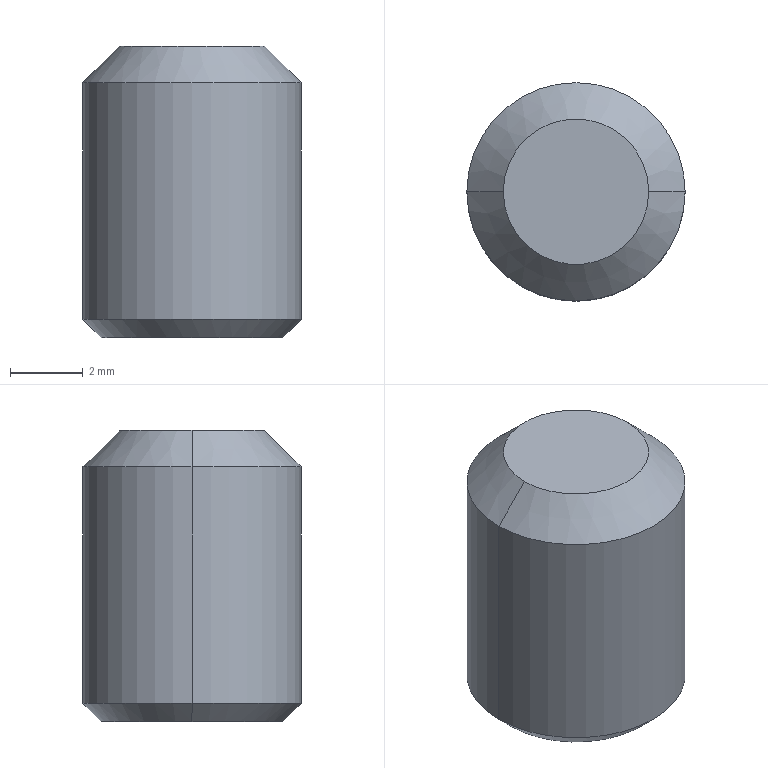Part | NX | features BREP 1 | 1 solid | 22 faces | box 6 x 6 x 8 mm | volume 197.963 mm3 | plane 14 | cone 6 | cylinder 2 | commonest cylinder face diameters 6 x2
STEP:
#1=CARTESIAN_POINT('',(0.,0.,2.866));
#2=VERTEX_POINT('',#1);
#3=CARTESIAN_POINT('',(-1.5,0.,2.));
#4=VERTEX_POINT('',#3);
#5=CARTESIAN_POINT('',(-1.5,0.,2.));
#6=DIRECTION('',(-0.866,0.,-0.5));
#7=VECTOR('',#6,1000.);
#8=LINE('',#5,#7);
#9=EDGE_CURVE('',#2,#4,#8,.T.);
#10=ORIENTED_EDGE('',*,*,#9,.F.);
#11=CARTESIAN_POINT('',(1.5,0.,2.));
#12=VERTEX_POINT('',#11);
#13=CARTESIAN_POINT('',(1.5,0.,2.));
#14=DIRECTION('',(0.866,0.,-0.5));
#15=VECTOR('',#14,1000.);
#16=LINE('',#13,#15);
#17=EDGE_CURVE('',#2,#12,#16,.T.);
#18=ORIENTED_EDGE('',*,*,#17,.T.);
#19=CARTESIAN_POINT('',(1.299,-0.75,2.));
#20=VERTEX_POINT('',#19);
#21=CARTESIAN_POINT('',(0.,0.,2.));
#22=DIRECTION('',(0.,0.,-1.));
#23=DIRECTION('',(-1.,0.,0.));
#24=AXIS2_PLACEMENT_3D('',#21,#22,#23);
#25=CIRCLE('',#24,1.5);
#26=EDGE_CURVE('',#12,#20,#25,.T.);
#27=ORIENTED_EDGE('',*,*,#26,.T.);
#28=CARTESIAN_POINT('',(0.,-1.5,2.));
#29=VERTEX_POINT('',#28);
#30=CARTESIAN_POINT('',(0.,0.,2.));
#31=DIRECTION('',(0.,0.,-1.));
#32=DIRECTION('',(-1.,0.,0.));
#33=AXIS2_PLACEMENT_3D('',#30,#31,#32);
#34=CIRCLE('',#33,1.5);
#35=EDGE_CURVE('',#20,#29,#34,.T.);
#36=ORIENTED_EDGE('',*,*,#35,.T.);
#37=CARTESIAN_POINT('',(-1.299,-0.75,2.));
#38=VERTEX_POINT('',#37);
#39=CARTESIAN_POINT('',(0.,0.,2.));
#40=DIRECTION('',(0.,0.,-1.));
#41=DIRECTION('',(-1.,0.,0.));
#42=AXIS2_PLACEMENT_3D('',#39,#40,#41);
#43=CIRCLE('',#42,1.5);
#44=EDGE_CURVE('',#29,#38,#43,.T.);
#45=ORIENTED_EDGE('',*,*,#44,.T.);
#46=CARTESIAN_POINT('',(0.,0.,2.));
#47=DIRECTION('',(0.,0.,-1.));
#48=DIRECTION('',(-1.,0.,0.));
#49=AXIS2_PLACEMENT_3D('',#46,#47,#48);
#50=CIRCLE('',#49,1.5);
#51=EDGE_CURVE('',#38,#4,#50,.T.);
#52=ORIENTED_EDGE('',*,*,#51,.T.);
#53=EDGE_LOOP('',(#10,#18,#27,#36,#45,#52));
#54=FACE_BOUND('',#53,.T.);
#55=CARTESIAN_POINT('',(0.,0.,2.));
#56=DIRECTION('',(0.,0.,-1.));
#57=DIRECTION('',(-1.,0.,0.));
#58=AXIS2_PLACEMENT_3D('',#55,#56,#57);
#59=CONICAL_SURFACE('',#58,1.5,1.047);
#60=ADVANCED_FACE('',(#54),#59,.F.);
#61=CARTESIAN_POINT('',(2.,0.,8.));
#62=VERTEX_POINT('',#61);
#63=CARTESIAN_POINT('',(-2.,0.,8.));
#64=VERTEX_POINT('',#63);
#65=CARTESIAN_POINT('',(0.,0.,8.));
#66=DIRECTION('',(0.,0.,1.));
#67=DIRECTION('',(1.,0.,0.));
#68=AXIS2_PLACEMENT_3D('',#65,#66,#67);
#69=CIRCLE('',#68,2.);
#70=EDGE_CURVE('',#62,#64,#69,.T.);
#71=ORIENTED_EDGE('',*,*,#70,.F.);
#72=CARTESIAN_POINT('',(3.,0.,7.));
#73=VERTEX_POINT('',#72);
#74=CARTESIAN_POINT('',(2.,0.,8.));
#75=DIRECTION('',(0.7071,0.,-0.7071));
#76=VECTOR('',#75,1000.);
#77=LINE('',#74,#76);
#78=EDGE_CURVE('',#62,#73,#77,.T.);
#79=ORIENTED_EDGE('',*,*,#78,.T.);
#80=CARTESIAN_POINT('',(-3.,0.,7.));
#81=VERTEX_POINT('',#80);
#82=CARTESIAN_POINT('',(0.,0.,7.));
#83=DIRECTION('',(0.,0.,-1.));
#84=DIRECTION('',(1.,0.,0.));
#85=AXIS2_PLACEMENT_3D('',#82,#83,#84);
#86=CIRCLE('',#85,3.);
#87=EDGE_CURVE('',#81,#73,#86,.T.);
#88=ORIENTED_EDGE('',*,*,#87,.F.);
#89=CARTESIAN_POINT('',(-2.,0.,8.));
#90=DIRECTION('',(-0.7071,0.,-0.7071));
#91=VECTOR('',#90,1000.);
#92=LINE('',#89,#91);
#93=EDGE_CURVE('',#64,#81,#92,.T.);
#94=ORIENTED_EDGE('',*,*,#93,.F.);
#95=EDGE_LOOP('',(#71,#79,#88,#94));
#96=FACE_BOUND('',#95,.T.);
#97=CARTESIAN_POINT('',(0.,0.,8.));
#98=DIRECTION('',(0.,0.,-1.));
#99=DIRECTION('',(-1.,0.,0.));
#100=AXIS2_PLACEMENT_3D('',#97,#98,#99);
#101=CONICAL_SURFACE('',#100,2.,0.7854);
#102=ADVANCED_FACE('',(#96),#101,.T.);
#103=CARTESIAN_POINT('',(-2.5,0.,0.));
#104=VERTEX_POINT('',#103);
#105=CARTESIAN_POINT('',(2.5,0.,0.));
#106=VERTEX_POINT('',#105);
#107=CARTESIAN_POINT('',(0.,0.,0.));
#108=DIRECTION('',(0.,0.,-1.));
#109=DIRECTION('',(1.,0.,0.));
#110=AXIS2_PLACEMENT_3D('',#107,#108,#109);
#111=CIRCLE('',#110,2.5);
#112=EDGE_CURVE('',#104,#106,#111,.T.);
#113=ORIENTED_EDGE('',*,*,#112,.F.);
#114=CARTESIAN_POINT('',(-3.,0.,0.5));
#115=VERTEX_POINT('',#114);
#116=CARTESIAN_POINT('',(-3.,0.,0.5));
#117=DIRECTION('',(-0.7071,0.,0.7071));
#118=VECTOR('',#117,1000.);
#119=LINE('',#116,#118);
#120=EDGE_CURVE('',#115,#104,#119,.F.);
#121=ORIENTED_EDGE('',*,*,#120,.F.);
#122=CARTESIAN_POINT('',(3.,0.,0.5));
#123=VERTEX_POINT('',#122);
#124=CARTESIAN_POINT('',(0.,0.,0.5));
#125=DIRECTION('',(0.,0.,1.));
#126=DIRECTION('',(1.,0.,0.));
#127=AXIS2_PLACEMENT_3D('',#124,#125,#126);
#128=CIRCLE('',#127,3.);
#129=EDGE_CURVE('',#123,#115,#128,.T.);
#130=ORIENTED_EDGE('',*,*,#129,.F.);
#131=CARTESIAN_POINT('',(3.,0.,0.5));
#132=DIRECTION('',(0.7071,0.,0.7071));
#133=VECTOR('',#132,1000.);
#134=LINE('',#131,#133);
#135=EDGE_CURVE('',#123,#106,#134,.F.);
#136=ORIENTED_EDGE('',*,*,#135,.T.);
#137=EDGE_LOOP('',(#113,#121,#130,#136));
#138=FACE_BOUND('',#137,.T.);
#139=CARTESIAN_POINT('',(0.,0.,0.5));
#140=DIRECTION('',(0.,0.,1.));
#141=DIRECTION('',(1.,0.,0.));
#142=AXIS2_PLACEMENT_3D('',#139,#140,#141);
#143=CONICAL_SURFACE('',#142,3.,0.7854);
#144=ADVANCED_FACE('',(#138),#143,.T.);
#145=ORIENTED_EDGE('',*,*,#87,.T.);
#146=CARTESIAN_POINT('',(3.,0.,8.));
#147=DIRECTION('',(0.,0.,-1.));
#148=VECTOR('',#147,1000.);
#149=LINE('',#146,#148);
#150=EDGE_CURVE('',#73,#123,#149,.T.);
#151=ORIENTED_EDGE('',*,*,#150,.T.);
#152=ORIENTED_EDGE('',*,*,#129,.T.);
#153=CARTESIAN_POINT('',(-3.,0.,8.));
#154=DIRECTION('',(0.,0.,-1.));
#155=VECTOR('',#154,1000.);
#156=LINE('',#153,#155);
#157=EDGE_CURVE('',#81,#115,#156,.T.);
#158=ORIENTED_EDGE('',*,*,#157,.F.);
#159=EDGE_LOOP('',(#145,#151,#152,#158));
#160=FACE_BOUND('',#159,.T.);
#161=CARTESIAN_POINT('',(0.,0.,8.));
#162=DIRECTION('',(0.,0.,-1.));
#163=DIRECTION('',(-1.,0.,0.));
#164=AXIS2_PLACEMENT_3D('',#161,#162,#163);
#165=CYLINDRICAL_SURFACE('',#164,3.);
#166=ADVANCED_FACE('',(#160),#165,.T.);
#167=CARTESIAN_POINT('',(-1.299,0.75,2.));
#168=VERTEX_POINT('',#167);
#169=CARTESIAN_POINT('',(0.,1.5,2.));
#170=VERTEX_POINT('',#169);
#171=CARTESIAN_POINT('',(0.,0.,2.));
#172=DIRECTION('',(0.,0.,-1.));
#173=DIRECTION('',(-1.,0.,0.));
#174=AXIS2_PLACEMENT_3D('',#171,#172,#173);
#175=CIRCLE('',#174,1.5);
#176=EDGE_CURVE('',#168,#170,#175,.T.);
#177=ORIENTED_EDGE('',*,*,#176,.F.);
#178=CARTESIAN_POINT('',(-0.866,1.5,2.));
#179=VERTEX_POINT('',#178);
#180=CARTESIAN_POINT('',(-1.732,0.,2.));
#181=DIRECTION('',(0.5,0.866,0.));
#182=VECTOR('',#181,1000.);
#183=LINE('',#180,#182);
#184=EDGE_CURVE('',#168,#179,#183,.T.);
#185=ORIENTED_EDGE('',*,*,#184,.T.);
#186=CARTESIAN_POINT('',(-0.866,1.5,2.));
#187=DIRECTION('',(1.,0.,0.));
#188=VECTOR('',#187,1000.);
#189=LINE('',#186,#188);
#190=EDGE_CURVE('',#179,#170,#189,.T.);
#191=ORIENTED_EDGE('',*,*,#190,.T.);
#192=EDGE_LOOP('',(#177,#185,#191));
#193=FACE_BOUND('',#192,.T.);
#194=CARTESIAN_POINT('',(0.,0.,2.));
#195=DIRECTION('',(0.,0.,-1.));
#196=DIRECTION('',(0.,-1.,0.));
#197=AXIS2_PLACEMENT_3D('',#194,#195,#196);
#198=PLANE('',#197);
#199=ADVANCED_FACE('',(#193),#198,.T.);
#200=CARTESIAN_POINT('',(1.299,0.75,2.));
#201=VERTEX_POINT('',#200);
#202=CARTESIAN_POINT('',(0.,0.,2.));
#203=DIRECTION('',(0.,0.,-1.));
#204=DIRECTION('',(-1.,0.,0.));
#205=AXIS2_PLACEMENT_3D('',#202,#203,#204);
#206=CIRCLE('',#205,1.5);
#207=EDGE_CURVE('',#170,#201,#206,.T.);
#208=ORIENTED_EDGE('',*,*,#207,.F.);
#209=CARTESIAN_POINT('',(0.866,1.5,2.));
#210=VERTEX_POINT('',#209);
#211=CARTESIAN_POINT('',(-0.866,1.5,2.));
#212=DIRECTION('',(1.,0.,0.));
#213=VECTOR('',#212,1000.);
#214=LINE('',#211,#213);
#215=EDGE_CURVE('',#170,#210,#214,.T.);
#216=ORIENTED_EDGE('',*,*,#215,.T.);
#217=CARTESIAN_POINT('',(0.866,1.5,2.));
#218=DIRECTION('',(0.5,-0.866,0.));
#219=VECTOR('',#218,1000.);
#220=LINE('',#217,#219);
#221=EDGE_CURVE('',#210,#201,#220,.T.);
#222=ORIENTED_EDGE('',*,*,#221,.T.);
#223=EDGE_LOOP('',(#208,#216,#222));
#224=FACE_BOUND('',#223,.T.);
#225=CARTESIAN_POINT('',(0.,0.,2.));
#226=DIRECTION('',(0.,0.,-1.));
#227=DIRECTION('',(0.,-1.,0.));
#228=AXIS2_PLACEMENT_3D('',#225,#226,#227);
#229=PLANE('',#228);
#230=ADVANCED_FACE('',(#224),#229,.T.);
#231=CARTESIAN_POINT('',(0.,0.,2.));
#232=DIRECTION('',(0.,0.,-1.));
#233=DIRECTION('',(-1.,0.,0.));
#234=AXIS2_PLACEMENT_3D('',#231,#232,#233);
#235=CIRCLE('',#234,1.5);
#236=EDGE_CURVE('',#201,#12,#235,.T.);
#237=ORIENTED_EDGE('',*,*,#236,.F.);
#238=CARTESIAN_POINT('',(1.732,0.,2.));
#239=VERTEX_POINT('',#238);
#240=CARTESIAN_POINT('',(0.866,1.5,2.));
#241=DIRECTION('',(0.5,-0.866,0.));
#242=VECTOR('',#241,1000.);
#243=LINE('',#240,#242);
#244=EDGE_CURVE('',#201,#239,#243,.T.);
#245=ORIENTED_EDGE('',*,*,#244,.T.);
#246=CARTESIAN_POINT('',(1.732,0.,2.));
#247=DIRECTION('',(-0.5,-0.866,0.));
#248=VECTOR('',#247,1000.);
#249=LINE('',#246,#248);
#250=EDGE_CURVE('',#239,#20,#249,.T.);
#251=ORIENTED_EDGE('',*,*,#250,.T.);
#252=ORIENTED_EDGE('',*,*,#26,.F.);
#253=EDGE_LOOP('',(#237,#245,#251,#252));
#254=FACE_BOUND('',#253,.T.);
#255=CARTESIAN_POINT('',(0.,0.,2.));
#256=DIRECTION('',(0.,0.,-1.));
#257=DIRECTION('',(0.,-1.,0.));
#258=AXIS2_PLACEMENT_3D('',#255,#256,#257);
#259=PLANE('',#258);
#260=ADVANCED_FACE('',(#254),#259,.T.);
#261=ORIENTED_EDGE('',*,*,#35,.F.);
#262=CARTESIAN_POINT('',(0.866,-1.5,2.));
#263=VERTEX_POINT('',#262);
#264=CARTESIAN_POINT('',(1.732,0.,2.));
#265=DIRECTION('',(-0.5,-0.866,0.));
#266=VECTOR('',#265,1000.);
#267=LINE('',#264,#266);
#268=EDGE_CURVE('',#20,#263,#267,.T.);
#269=ORIENTED_EDGE('',*,*,#268,.T.);
#270=CARTESIAN_POINT('',(0.866,-1.5,2.));
#271=DIRECTION('',(-1.,0.,0.));
#272=VECTOR('',#271,1000.);
#273=LINE('',#270,#272);
#274=EDGE_CURVE('',#263,#29,#273,.T.);
#275=ORIENTED_EDGE('',*,*,#274,.T.);
#276=EDGE_LOOP('',(#261,#269,#275));
#277=FACE_BOUND('',#276,.T.);
#278=CARTESIAN_POINT('',(0.,0.,2.));
#279=DIRECTION('',(0.,0.,-1.));
#280=DIRECTION('',(0.,-1.,0.));
#281=AXIS2_PLACEMENT_3D('',#278,#279,#280);
#282=PLANE('',#281);
#283=ADVANCED_FACE('',(#277),#282,.T.);
#284=ORIENTED_EDGE('',*,*,#44,.F.);
#285=CARTESIAN_POINT('',(-0.866,-1.5,2.));
#286=VERTEX_POINT('',#285);
#287=CARTESIAN_POINT('',(0.866,-1.5,2.));
#288=DIRECTION('',(-1.,0.,0.));
#289=VECTOR('',#288,1000.);
#290=LINE('',#287,#289);
#291=EDGE_CURVE('',#29,#286,#290,.T.);
#292=ORIENTED_EDGE('',*,*,#291,.T.);
#293=CARTESIAN_POINT('',(-0.866,-1.5,2.));
#294=DIRECTION('',(-0.5,0.866,0.));
#295=VECTOR('',#294,1000.);
#296=LINE('',#293,#295);
#297=EDGE_CURVE('',#286,#38,#296,.T.);
#298=ORIENTED_EDGE('',*,*,#297,.T.);
#299=EDGE_LOOP('',(#284,#292,#298));
#300=FACE_BOUND('',#299,.T.);
#301=CARTESIAN_POINT('',(0.,0.,2.));
#302=DIRECTION('',(0.,0.,-1.));
#303=DIRECTION('',(0.,-1.,0.));
#304=AXIS2_PLACEMENT_3D('',#301,#302,#303);
#305=PLANE('',#304);
#306=ADVANCED_FACE('',(#300),#305,.T.);
#307=ORIENTED_EDGE('',*,*,#150,.F.);
#308=CARTESIAN_POINT('',(0.,0.,7.));
#309=DIRECTION('',(0.,0.,-1.));
#310=DIRECTION('',(1.,0.,0.));
#311=AXIS2_PLACEMENT_3D('',#308,#309,#310);
#312=CIRCLE('',#311,3.);
#313=EDGE_CURVE('',#73,#81,#312,.T.);
#314=ORIENTED_EDGE('',*,*,#313,.T.);
#315=ORIENTED_EDGE('',*,*,#157,.T.);
#316=CARTESIAN_POINT('',(0.,0.,0.5));
#317=DIRECTION('',(0.,0.,1.));
#318=DIRECTION('',(1.,0.,0.));
#319=AXIS2_PLACEMENT_3D('',#316,#317,#318);
#320=CIRCLE('',#319,3.);
#321=EDGE_CURVE('',#115,#123,#320,.T.);
#322=ORIENTED_EDGE('',*,*,#321,.T.);
#323=EDGE_LOOP('',(#307,#314,#315,#322));
#324=FACE_BOUND('',#323,.T.);
#325=CARTESIAN_POINT('',(0.,0.,8.));
#326=DIRECTION('',(0.,0.,-1.));
#327=DIRECTION('',(-1.,0.,0.));
#328=AXIS2_PLACEMENT_3D('',#325,#326,#327);
#329=CYLINDRICAL_SURFACE('',#328,3.);
#330=ADVANCED_FACE('',(#324),#329,.T.);
#331=CARTESIAN_POINT('',(0.,0.,8.));
#332=DIRECTION('',(0.,0.,1.));
#333=DIRECTION('',(1.,0.,0.));
#334=AXIS2_PLACEMENT_3D('',#331,#332,#333);
#335=CIRCLE('',#334,2.);
#336=EDGE_CURVE('',#64,#62,#335,.T.);
#337=ORIENTED_EDGE('',*,*,#336,.T.);
#338=ORIENTED_EDGE('',*,*,#70,.T.);
#339=EDGE_LOOP('',(#337,#338));
#340=FACE_BOUND('',#339,.T.);
#341=CARTESIAN_POINT('',(0.,0.,8.));
#342=DIRECTION('',(0.,0.,1.));
#343=DIRECTION('',(1.,0.,0.));
#344=AXIS2_PLACEMENT_3D('',#341,#342,#343);
#345=PLANE('',#344);
#346=ADVANCED_FACE('',(#340),#345,.T.);
#347=CARTESIAN_POINT('',(0.,0.,0.));
#348=DIRECTION('',(0.,0.,-1.));
#349=DIRECTION('',(1.,0.,0.));
#350=AXIS2_PLACEMENT_3D('',#347,#348,#349);
#351=CIRCLE('',#350,2.5);
#352=EDGE_CURVE('',#106,#104,#351,.T.);
#353=ORIENTED_EDGE('',*,*,#352,.T.);
#354=ORIENTED_EDGE('',*,*,#112,.T.);
#355=EDGE_LOOP('',(#353,#354));
#356=FACE_BOUND('',#355,.T.);
#357=CARTESIAN_POINT('',(-0.866,1.5,0.));
#358=VERTEX_POINT('',#357);
#359=CARTESIAN_POINT('',(0.866,1.5,0.));
#360=VERTEX_POINT('',#359);
#361=CARTESIAN_POINT('',(-0.866,1.5,0.));
#362=DIRECTION('',(1.,0.,0.));
#363=VECTOR('',#362,1000.);
#364=LINE('',#361,#363);
#365=EDGE_CURVE('',#358,#360,#364,.T.);
#366=ORIENTED_EDGE('',*,*,#365,.F.);
#367=CARTESIAN_POINT('',(-1.732,0.,0.));
#368=VERTEX_POINT('',#367);
#369=CARTESIAN_POINT('',(-1.732,0.,0.));
#370=DIRECTION('',(0.5,0.866,0.));
#371=VECTOR('',#370,1000.);
#372=LINE('',#369,#371);
#373=EDGE_CURVE('',#368,#358,#372,.T.);
#374=ORIENTED_EDGE('',*,*,#373,.F.);
#375=CARTESIAN_POINT('',(-0.866,-1.5,0.));
#376=VERTEX_POINT('',#375);
#377=CARTESIAN_POINT('',(-0.866,-1.5,0.));
#378=DIRECTION('',(-0.5,0.866,0.));
#379=VECTOR('',#378,1000.);
#380=LINE('',#377,#379);
#381=EDGE_CURVE('',#376,#368,#380,.T.);
#382=ORIENTED_EDGE('',*,*,#381,.F.);
#383=CARTESIAN_POINT('',(0.866,-1.5,0.));
#384=VERTEX_POINT('',#383);
#385=CARTESIAN_POINT('',(0.866,-1.5,0.));
#386=DIRECTION('',(-1.,0.,0.));
#387=VECTOR('',#386,1000.);
#388=LINE('',#385,#387);
#389=EDGE_CURVE('',#384,#376,#388,.T.);
#390=ORIENTED_EDGE('',*,*,#389,.F.);
#391=CARTESIAN_POINT('',(1.732,0.,0.));
#392=VERTEX_POINT('',#391);
#393=CARTESIAN_POINT('',(1.732,0.,0.));
#394=DIRECTION('',(-0.5,-0.866,0.));
#395=VECTOR('',#394,1000.);
#396=LINE('',#393,#395);
#397=EDGE_CURVE('',#392,#384,#396,.T.);
#398=ORIENTED_EDGE('',*,*,#397,.F.);
#399=CARTESIAN_POINT('',(0.866,1.5,0.));
#400=DIRECTION('',(0.5,-0.866,0.));
#401=VECTOR('',#400,1000.);
#402=LINE('',#399,#401);
#403=EDGE_CURVE('',#360,#392,#402,.T.);
#404=ORIENTED_EDGE('',*,*,#403,.F.);
#405=EDGE_LOOP('',(#366,#374,#382,#390,#398,#404));
#406=FACE_BOUND('',#405,.T.);
#407=CARTESIAN_POINT('',(0.,0.,0.));
#408=DIRECTION('',(0.,0.,1.));
#409=DIRECTION('',(1.,0.,0.));
#410=AXIS2_PLACEMENT_3D('',#407,#408,#409);
#411=PLANE('',#410);
#412=ADVANCED_FACE('',(#356,#406),#411,.F.);
#413=ORIENTED_EDGE('',*,*,#120,.T.);
#414=ORIENTED_EDGE('',*,*,#352,.F.);
#415=ORIENTED_EDGE('',*,*,#135,.F.);
#416=ORIENTED_EDGE('',*,*,#321,.F.);
#417=EDGE_LOOP('',(#413,#414,#415,#416));
#418=FACE_BOUND('',#417,.T.);
#419=CARTESIAN_POINT('',(0.,0.,0.5));
#420=DIRECTION('',(0.,0.,1.));
#421=DIRECTION('',(1.,0.,0.));
#422=AXIS2_PLACEMENT_3D('',#419,#420,#421);
#423=CONICAL_SURFACE('',#422,3.,0.7854);
#424=ADVANCED_FACE('',(#418),#423,.T.);
#425=ORIENTED_EDGE('',*,*,#78,.F.);
#426=ORIENTED_EDGE('',*,*,#336,.F.);
#427=ORIENTED_EDGE('',*,*,#93,.T.);
#428=ORIENTED_EDGE('',*,*,#313,.F.);
#429=EDGE_LOOP('',(#425,#426,#427,#428));
#430=FACE_BOUND('',#429,.T.);
#431=CARTESIAN_POINT('',(0.,0.,8.));
#432=DIRECTION('',(0.,0.,-1.));
#433=DIRECTION('',(-1.,0.,0.));
#434=AXIS2_PLACEMENT_3D('',#431,#432,#433);
#435=CONICAL_SURFACE('',#434,2.,0.7854);
#436=ADVANCED_FACE('',(#430),#435,.T.);
#437=ORIENTED_EDGE('',*,*,#373,.T.);
#438=CARTESIAN_POINT('',(-0.866,1.5,2.));
#439=DIRECTION('',(0.,0.,-1.));
#440=VECTOR('',#439,1000.);
#441=LINE('',#438,#440);
#442=EDGE_CURVE('',#179,#358,#441,.T.);
#443=ORIENTED_EDGE('',*,*,#442,.F.);
#444=ORIENTED_EDGE('',*,*,#184,.F.);
#445=CARTESIAN_POINT('',(-1.732,0.,2.));
#446=VERTEX_POINT('',#445);
#447=CARTESIAN_POINT('',(-1.732,0.,2.));
#448=DIRECTION('',(0.5,0.866,0.));
#449=VECTOR('',#448,1000.);
#450=LINE('',#447,#449);
#451=EDGE_CURVE('',#446,#168,#450,.T.);
#452=ORIENTED_EDGE('',*,*,#451,.F.);
#453=CARTESIAN_POINT('',(-1.732,0.,2.));
#454=DIRECTION('',(0.,0.,-1.));
#455=VECTOR('',#454,1000.);
#456=LINE('',#453,#455);
#457=EDGE_CURVE('',#446,#368,#456,.T.);
#458=ORIENTED_EDGE('',*,*,#457,.T.);
#459=EDGE_LOOP('',(#437,#443,#444,#452,#458));
#460=FACE_BOUND('',#459,.T.);
#461=CARTESIAN_POINT('',(-1.732,0.,2.));
#462=DIRECTION('',(-0.866,0.5,0.));
#463=DIRECTION('',(0.,0.,1.));
#464=AXIS2_PLACEMENT_3D('',#461,#462,#463);
#465=PLANE('',#464);
#466=ADVANCED_FACE('',(#460),#465,.F.);
#467=ORIENTED_EDGE('',*,*,#381,.T.);
#468=ORIENTED_EDGE('',*,*,#457,.F.);
#469=CARTESIAN_POINT('',(-0.866,-1.5,2.));
#470=DIRECTION('',(-0.5,0.866,0.));
#471=VECTOR('',#470,1000.);
#472=LINE('',#469,#471);
#473=EDGE_CURVE('',#38,#446,#472,.T.);
#474=ORIENTED_EDGE('',*,*,#473,.F.);
#475=ORIENTED_EDGE('',*,*,#297,.F.);
#476=CARTESIAN_POINT('',(-0.866,-1.5,2.));
#477=DIRECTION('',(0.,0.,-1.));
#478=VECTOR('',#477,1000.);
#479=LINE('',#476,#478);
#480=EDGE_CURVE('',#286,#376,#479,.T.);
#481=ORIENTED_EDGE('',*,*,#480,.T.);
#482=EDGE_LOOP('',(#467,#468,#474,#475,#481));
#483=FACE_BOUND('',#482,.T.);
#484=CARTESIAN_POINT('',(-0.866,-1.5,2.));
#485=DIRECTION('',(-0.866,-0.5,0.));
#486=DIRECTION('',(-0.5,0.866,0.));
#487=AXIS2_PLACEMENT_3D('',#484,#485,#486);
#488=PLANE('',#487);
#489=ADVANCED_FACE('',(#483),#488,.F.);
#490=ORIENTED_EDGE('',*,*,#389,.T.);
#491=ORIENTED_EDGE('',*,*,#480,.F.);
#492=ORIENTED_EDGE('',*,*,#291,.F.);
#493=ORIENTED_EDGE('',*,*,#274,.F.);
#494=CARTESIAN_POINT('',(0.866,-1.5,2.));
#495=DIRECTION('',(0.,0.,-1.));
#496=VECTOR('',#495,1000.);
#497=LINE('',#494,#496);
#498=EDGE_CURVE('',#263,#384,#497,.T.);
#499=ORIENTED_EDGE('',*,*,#498,.T.);
#500=EDGE_LOOP('',(#490,#491,#492,#493,#499));
#501=FACE_BOUND('',#500,.T.);
#502=CARTESIAN_POINT('',(0.866,-1.5,2.));
#503=DIRECTION('',(0.,-1.,0.));
#504=DIRECTION('',(0.,0.,-1.));
#505=AXIS2_PLACEMENT_3D('',#502,#503,#504);
#506=PLANE('',#505);
#507=ADVANCED_FACE('',(#501),#506,.F.);
#508=ORIENTED_EDGE('',*,*,#397,.T.);
#509=ORIENTED_EDGE('',*,*,#498,.F.);
#510=ORIENTED_EDGE('',*,*,#268,.F.);
#511=ORIENTED_EDGE('',*,*,#250,.F.);
#512=CARTESIAN_POINT('',(1.732,0.,2.));
#513=DIRECTION('',(0.,0.,-1.));
#514=VECTOR('',#513,1000.);
#515=LINE('',#512,#514);
#516=EDGE_CURVE('',#239,#392,#515,.T.);
#517=ORIENTED_EDGE('',*,*,#516,.T.);
#518=EDGE_LOOP('',(#508,#509,#510,#511,#517));
#519=FACE_BOUND('',#518,.T.);
#520=CARTESIAN_POINT('',(1.732,0.,2.));
#521=DIRECTION('',(0.866,-0.5,0.));
#522=DIRECTION('',(0.,0.,-1.));
#523=AXIS2_PLACEMENT_3D('',#520,#521,#522);
#524=PLANE('',#523);
#525=ADVANCED_FACE('',(#519),#524,.F.);
#526=ORIENTED_EDGE('',*,*,#403,.T.);
#527=ORIENTED_EDGE('',*,*,#516,.F.);
#528=ORIENTED_EDGE('',*,*,#244,.F.);
#529=ORIENTED_EDGE('',*,*,#221,.F.);
#530=CARTESIAN_POINT('',(0.866,1.5,2.));
#531=DIRECTION('',(0.,0.,-1.));
#532=VECTOR('',#531,1000.);
#533=LINE('',#530,#532);
#534=EDGE_CURVE('',#210,#360,#533,.T.);
#535=ORIENTED_EDGE('',*,*,#534,.T.);
#536=EDGE_LOOP('',(#526,#527,#528,#529,#535));
#537=FACE_BOUND('',#536,.T.);
#538=CARTESIAN_POINT('',(0.866,1.5,2.));
#539=DIRECTION('',(0.866,0.5,0.));
#540=DIRECTION('',(0.,0.,-1.));
#541=AXIS2_PLACEMENT_3D('',#538,#539,#540);
#542=PLANE('',#541);
#543=ADVANCED_FACE('',(#537),#542,.F.);
#544=ORIENTED_EDGE('',*,*,#365,.T.);
#545=ORIENTED_EDGE('',*,*,#534,.F.);
#546=ORIENTED_EDGE('',*,*,#215,.F.);
#547=ORIENTED_EDGE('',*,*,#190,.F.);
#548=ORIENTED_EDGE('',*,*,#442,.T.);
#549=EDGE_LOOP('',(#544,#545,#546,#547,#548));
#550=FACE_BOUND('',#549,.T.);
#551=CARTESIAN_POINT('',(-0.866,1.5,2.));
#552=DIRECTION('',(0.,1.,0.));
#553=DIRECTION('',(1.,0.,0.));
#554=AXIS2_PLACEMENT_3D('',#551,#552,#553);
#555=PLANE('',#554);
#556=ADVANCED_FACE('',(#550),#555,.F.);
#557=ORIENTED_EDGE('',*,*,#51,.F.);
#558=ORIENTED_EDGE('',*,*,#473,.T.);
#559=ORIENTED_EDGE('',*,*,#451,.T.);
#560=CARTESIAN_POINT('',(0.,0.,2.));
#561=DIRECTION('',(0.,0.,-1.));
#562=DIRECTION('',(-1.,0.,0.));
#563=AXIS2_PLACEMENT_3D('',#560,#561,#562);
#564=CIRCLE('',#563,1.5);
#565=EDGE_CURVE('',#4,#168,#564,.T.);
#566=ORIENTED_EDGE('',*,*,#565,.F.);
#567=EDGE_LOOP('',(#557,#558,#559,#566));
#568=FACE_BOUND('',#567,.T.);
#569=CARTESIAN_POINT('',(0.,0.,2.));
#570=DIRECTION('',(0.,0.,-1.));
#571=DIRECTION('',(0.,-1.,0.));
#572=AXIS2_PLACEMENT_3D('',#569,#570,#571);
#573=PLANE('',#572);
#574=ADVANCED_FACE('',(#568),#573,.T.);
#575=ORIENTED_EDGE('',*,*,#17,.F.);
#576=ORIENTED_EDGE('',*,*,#9,.T.);
#577=ORIENTED_EDGE('',*,*,#565,.T.);
#578=ORIENTED_EDGE('',*,*,#176,.T.);
#579=ORIENTED_EDGE('',*,*,#207,.T.);
#580=ORIENTED_EDGE('',*,*,#236,.T.);
#581=EDGE_LOOP('',(#575,#576,#577,#578,#579,#580));
#582=FACE_BOUND('',#581,.T.);
#583=CARTESIAN_POINT('',(0.,0.,2.));
#584=DIRECTION('',(0.,0.,-1.));
#585=DIRECTION('',(-1.,0.,0.));
#586=AXIS2_PLACEMENT_3D('',#583,#584,#585);
#587=CONICAL_SURFACE('',#586,1.5,1.047);
#588=ADVANCED_FACE('',(#582),#587,.F.);
#589=CLOSED_SHELL('',(#60,#102,#144,#166,#199,#230,#260,#283,#306,#330,#346,#412,#424,#436,#466,#489,#507,#525,#543,#556,#574,#588));
#590=MANIFOLD_SOLID_BREP('',#589);
#591=(LENGTH_UNIT()NAMED_UNIT(*)SI_UNIT(.MILLI.,.METRE.));
#592=UNCERTAINTY_MEASURE_WITH_UNIT(LENGTH_MEASURE(0.00001),#591,'','');
#593=(NAMED_UNIT(*)PLANE_ANGLE_UNIT()SI_UNIT($,.RADIAN.));
#594=(NAMED_UNIT(*)SI_UNIT($,.STERADIAN.)SOLID_ANGLE_UNIT());
#595=(GEOMETRIC_REPRESENTATION_CONTEXT(3)GLOBAL_UNCERTAINTY_ASSIGNED_CONTEXT((#592))GLOBAL_UNIT_ASSIGNED_CONTEXT((#591,#593,#594))REPRESENTATION_CONTEXT('',''));
#596=ADVANCED_BREP_SHAPE_REPRESENTATION('',(#590),#595);